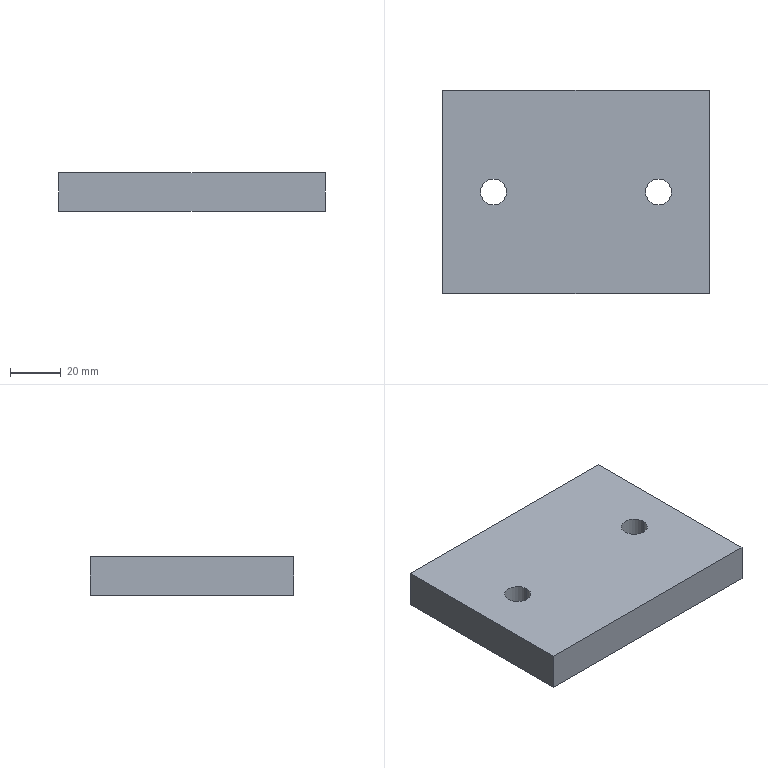Part | SolidWorks | features Extrusion 1, HoleWzd 1 | 1 solid | 10 faces | box 105 x 80 x 15 mm | volume 123549 mm3 | plane 6 | cylinder 4 | commonest cylinder face diameters 10.2 x4
STEP:
#1=CARTESIAN_POINT('',(-27.4,0.,0.));
#2=VERTEX_POINT('',#1);
#3=CARTESIAN_POINT('',(-37.6,0.,0.));
#4=VERTEX_POINT('',#3);
#5=CARTESIAN_POINT('',(-32.5,0.,0.));
#6=DIRECTION('',(0.,0.,-1.));
#7=DIRECTION('',(-1.,0.,0.));
#8=AXIS2_PLACEMENT_3D('',#5,#6,#7);
#9=CIRCLE('',#8,5.1);
#10=EDGE_CURVE('',#2,#4,#9,.T.);
#11=ORIENTED_EDGE('',*,*,#10,.T.);
#12=CARTESIAN_POINT('',(-37.6,0.,15.));
#13=VERTEX_POINT('',#12);
#14=CARTESIAN_POINT('',(-37.6,0.,15.));
#15=DIRECTION('',(0.,0.,1.));
#16=VECTOR('',#15,1000.);
#17=LINE('',#14,#16);
#18=EDGE_CURVE('',#4,#13,#17,.T.);
#19=ORIENTED_EDGE('',*,*,#18,.T.);
#20=CARTESIAN_POINT('',(-27.4,0.,15.));
#21=VERTEX_POINT('',#20);
#22=CARTESIAN_POINT('',(-32.5,0.,15.));
#23=DIRECTION('',(0.,0.,1.));
#24=DIRECTION('',(1.,0.,0.));
#25=AXIS2_PLACEMENT_3D('',#22,#23,#24);
#26=CIRCLE('',#25,5.1);
#27=EDGE_CURVE('',#13,#21,#26,.T.);
#28=ORIENTED_EDGE('',*,*,#27,.T.);
#29=CARTESIAN_POINT('',(-27.4,0.,15.));
#30=DIRECTION('',(0.,0.,1.));
#31=VECTOR('',#30,1000.);
#32=LINE('',#29,#31);
#33=EDGE_CURVE('',#2,#21,#32,.T.);
#34=ORIENTED_EDGE('',*,*,#33,.F.);
#35=EDGE_LOOP('',(#11,#19,#28,#34));
#36=FACE_OUTER_BOUND('',#35,.T.);
#37=CARTESIAN_POINT('',(-32.5,0.,15.));
#38=DIRECTION('',(0.,0.,1.));
#39=DIRECTION('',(1.,0.,0.));
#40=AXIS2_PLACEMENT_3D('',#37,#38,#39);
#41=CYLINDRICAL_SURFACE('',#40,5.1);
#42=ADVANCED_FACE('',(#36),#41,.F.);
#43=CARTESIAN_POINT('',(37.6,0.,0.));
#44=VERTEX_POINT('',#43);
#45=CARTESIAN_POINT('',(27.4,0.,0.));
#46=VERTEX_POINT('',#45);
#47=CARTESIAN_POINT('',(32.5,0.,0.));
#48=DIRECTION('',(0.,0.,-1.));
#49=DIRECTION('',(-1.,0.,0.));
#50=AXIS2_PLACEMENT_3D('',#47,#48,#49);
#51=CIRCLE('',#50,5.1);
#52=EDGE_CURVE('',#44,#46,#51,.T.);
#53=ORIENTED_EDGE('',*,*,#52,.T.);
#54=CARTESIAN_POINT('',(27.4,0.,15.));
#55=VERTEX_POINT('',#54);
#56=CARTESIAN_POINT('',(27.4,0.,15.));
#57=DIRECTION('',(0.,0.,1.));
#58=VECTOR('',#57,1000.);
#59=LINE('',#56,#58);
#60=EDGE_CURVE('',#46,#55,#59,.T.);
#61=ORIENTED_EDGE('',*,*,#60,.T.);
#62=CARTESIAN_POINT('',(37.6,0.,15.));
#63=VERTEX_POINT('',#62);
#64=CARTESIAN_POINT('',(32.5,0.,15.));
#65=DIRECTION('',(0.,0.,1.));
#66=DIRECTION('',(1.,0.,0.));
#67=AXIS2_PLACEMENT_3D('',#64,#65,#66);
#68=CIRCLE('',#67,5.1);
#69=EDGE_CURVE('',#55,#63,#68,.T.);
#70=ORIENTED_EDGE('',*,*,#69,.T.);
#71=CARTESIAN_POINT('',(37.6,0.,15.));
#72=DIRECTION('',(0.,0.,1.));
#73=VECTOR('',#72,1000.);
#74=LINE('',#71,#73);
#75=EDGE_CURVE('',#44,#63,#74,.T.);
#76=ORIENTED_EDGE('',*,*,#75,.F.);
#77=EDGE_LOOP('',(#53,#61,#70,#76));
#78=FACE_OUTER_BOUND('',#77,.T.);
#79=CARTESIAN_POINT('',(32.5,0.,15.));
#80=DIRECTION('',(0.,0.,1.));
#81=DIRECTION('',(1.,0.,0.));
#82=AXIS2_PLACEMENT_3D('',#79,#80,#81);
#83=CYLINDRICAL_SURFACE('',#82,5.1);
#84=ADVANCED_FACE('',(#78),#83,.F.);
#85=CARTESIAN_POINT('',(-52.5,40.,0.));
#86=VERTEX_POINT('',#85);
#87=CARTESIAN_POINT('',(-52.5,-40.,0.));
#88=VERTEX_POINT('',#87);
#89=CARTESIAN_POINT('',(-52.5,40.,0.));
#90=DIRECTION('',(0.,-1.,0.));
#91=VECTOR('',#90,1000.);
#92=LINE('',#89,#91);
#93=EDGE_CURVE('',#86,#88,#92,.T.);
#94=ORIENTED_EDGE('',*,*,#93,.T.);
#95=CARTESIAN_POINT('',(-52.5,-40.,15.));
#96=VERTEX_POINT('',#95);
#97=CARTESIAN_POINT('',(-52.5,-40.,15.));
#98=DIRECTION('',(0.,0.,-1.));
#99=VECTOR('',#98,1000.);
#100=LINE('',#97,#99);
#101=EDGE_CURVE('',#96,#88,#100,.T.);
#102=ORIENTED_EDGE('',*,*,#101,.F.);
#103=CARTESIAN_POINT('',(-52.5,40.,15.));
#104=VERTEX_POINT('',#103);
#105=CARTESIAN_POINT('',(-52.5,40.,15.));
#106=DIRECTION('',(0.,-1.,0.));
#107=VECTOR('',#106,1000.);
#108=LINE('',#105,#107);
#109=EDGE_CURVE('',#104,#96,#108,.T.);
#110=ORIENTED_EDGE('',*,*,#109,.F.);
#111=CARTESIAN_POINT('',(-52.5,40.,15.));
#112=DIRECTION('',(0.,0.,-1.));
#113=VECTOR('',#112,1000.);
#114=LINE('',#111,#113);
#115=EDGE_CURVE('',#104,#86,#114,.T.);
#116=ORIENTED_EDGE('',*,*,#115,.T.);
#117=EDGE_LOOP('',(#94,#102,#110,#116));
#118=FACE_OUTER_BOUND('',#117,.T.);
#119=CARTESIAN_POINT('',(-52.5,40.,15.));
#120=DIRECTION('',(1.,0.,0.));
#121=DIRECTION('',(0.,0.,-1.));
#122=AXIS2_PLACEMENT_3D('',#119,#120,#121);
#123=PLANE('',#122);
#124=ADVANCED_FACE('',(#118),#123,.F.);
#125=CARTESIAN_POINT('',(52.5,-40.,0.));
#126=VERTEX_POINT('',#125);
#127=CARTESIAN_POINT('',(52.5,-40.,0.));
#128=DIRECTION('',(1.,0.,0.));
#129=VECTOR('',#128,1000.);
#130=LINE('',#127,#129);
#131=EDGE_CURVE('',#88,#126,#130,.T.);
#132=ORIENTED_EDGE('',*,*,#131,.T.);
#133=CARTESIAN_POINT('',(52.5,-40.,15.));
#134=VERTEX_POINT('',#133);
#135=CARTESIAN_POINT('',(52.5,-40.,15.));
#136=DIRECTION('',(0.,0.,-1.));
#137=VECTOR('',#136,1000.);
#138=LINE('',#135,#137);
#139=EDGE_CURVE('',#134,#126,#138,.T.);
#140=ORIENTED_EDGE('',*,*,#139,.F.);
#141=CARTESIAN_POINT('',(52.5,-40.,15.));
#142=DIRECTION('',(1.,0.,0.));
#143=VECTOR('',#142,1000.);
#144=LINE('',#141,#143);
#145=EDGE_CURVE('',#96,#134,#144,.T.);
#146=ORIENTED_EDGE('',*,*,#145,.F.);
#147=ORIENTED_EDGE('',*,*,#101,.T.);
#148=EDGE_LOOP('',(#132,#140,#146,#147));
#149=FACE_OUTER_BOUND('',#148,.T.);
#150=CARTESIAN_POINT('',(52.5,-40.,15.));
#151=DIRECTION('',(0.,1.,0.));
#152=DIRECTION('',(-1.,0.,0.));
#153=AXIS2_PLACEMENT_3D('',#150,#151,#152);
#154=PLANE('',#153);
#155=ADVANCED_FACE('',(#149),#154,.F.);
#156=CARTESIAN_POINT('',(52.5,40.,0.));
#157=VERTEX_POINT('',#156);
#158=CARTESIAN_POINT('',(52.5,40.,0.));
#159=DIRECTION('',(0.,1.,0.));
#160=VECTOR('',#159,1000.);
#161=LINE('',#158,#160);
#162=EDGE_CURVE('',#126,#157,#161,.T.);
#163=ORIENTED_EDGE('',*,*,#162,.T.);
#164=CARTESIAN_POINT('',(52.5,40.,15.));
#165=VERTEX_POINT('',#164);
#166=CARTESIAN_POINT('',(52.5,40.,15.));
#167=DIRECTION('',(0.,0.,-1.));
#168=VECTOR('',#167,1000.);
#169=LINE('',#166,#168);
#170=EDGE_CURVE('',#165,#157,#169,.T.);
#171=ORIENTED_EDGE('',*,*,#170,.F.);
#172=CARTESIAN_POINT('',(52.5,40.,15.));
#173=DIRECTION('',(0.,1.,0.));
#174=VECTOR('',#173,1000.);
#175=LINE('',#172,#174);
#176=EDGE_CURVE('',#134,#165,#175,.T.);
#177=ORIENTED_EDGE('',*,*,#176,.F.);
#178=ORIENTED_EDGE('',*,*,#139,.T.);
#179=EDGE_LOOP('',(#163,#171,#177,#178));
#180=FACE_OUTER_BOUND('',#179,.T.);
#181=CARTESIAN_POINT('',(52.5,40.,15.));
#182=DIRECTION('',(-1.,0.,0.));
#183=DIRECTION('',(0.,-1.,0.));
#184=AXIS2_PLACEMENT_3D('',#181,#182,#183);
#185=PLANE('',#184);
#186=ADVANCED_FACE('',(#180),#185,.F.);
#187=CARTESIAN_POINT('',(52.5,40.,0.));
#188=DIRECTION('',(-1.,0.,0.));
#189=VECTOR('',#188,1000.);
#190=LINE('',#187,#189);
#191=EDGE_CURVE('',#157,#86,#190,.T.);
#192=ORIENTED_EDGE('',*,*,#191,.T.);
#193=ORIENTED_EDGE('',*,*,#115,.F.);
#194=CARTESIAN_POINT('',(52.5,40.,15.));
#195=DIRECTION('',(-1.,0.,0.));
#196=VECTOR('',#195,1000.);
#197=LINE('',#194,#196);
#198=EDGE_CURVE('',#165,#104,#197,.T.);
#199=ORIENTED_EDGE('',*,*,#198,.F.);
#200=ORIENTED_EDGE('',*,*,#170,.T.);
#201=EDGE_LOOP('',(#192,#193,#199,#200));
#202=FACE_OUTER_BOUND('',#201,.T.);
#203=CARTESIAN_POINT('',(52.5,40.,15.));
#204=DIRECTION('',(0.,-1.,0.));
#205=DIRECTION('',(1.,0.,0.));
#206=AXIS2_PLACEMENT_3D('',#203,#204,#205);
#207=PLANE('',#206);
#208=ADVANCED_FACE('',(#202),#207,.F.);
#209=CARTESIAN_POINT('',(-32.5,0.,15.));
#210=DIRECTION('',(0.,0.,1.));
#211=DIRECTION('',(1.,0.,0.));
#212=AXIS2_PLACEMENT_3D('',#209,#210,#211);
#213=CIRCLE('',#212,5.1);
#214=EDGE_CURVE('',#21,#13,#213,.T.);
#215=ORIENTED_EDGE('',*,*,#214,.F.);
#216=ORIENTED_EDGE('',*,*,#27,.F.);
#217=EDGE_LOOP('',(#215,#216));
#218=FACE_BOUND('',#217,.T.);
#219=CARTESIAN_POINT('',(32.5,0.,15.));
#220=DIRECTION('',(0.,0.,1.));
#221=DIRECTION('',(1.,0.,0.));
#222=AXIS2_PLACEMENT_3D('',#219,#220,#221);
#223=CIRCLE('',#222,5.1);
#224=EDGE_CURVE('',#63,#55,#223,.T.);
#225=ORIENTED_EDGE('',*,*,#224,.F.);
#226=ORIENTED_EDGE('',*,*,#69,.F.);
#227=EDGE_LOOP('',(#225,#226));
#228=FACE_BOUND('',#227,.T.);
#229=ORIENTED_EDGE('',*,*,#109,.T.);
#230=ORIENTED_EDGE('',*,*,#145,.T.);
#231=ORIENTED_EDGE('',*,*,#176,.T.);
#232=ORIENTED_EDGE('',*,*,#198,.T.);
#233=EDGE_LOOP('',(#229,#230,#231,#232));
#234=FACE_OUTER_BOUND('',#233,.T.);
#235=CARTESIAN_POINT('',(0.,0.,15.));
#236=DIRECTION('',(0.,0.,-1.));
#237=DIRECTION('',(-1.,0.,0.));
#238=AXIS2_PLACEMENT_3D('',#235,#236,#237);
#239=PLANE('',#238);
#240=ADVANCED_FACE('',(#218,#228,#234),#239,.F.);
#241=ORIENTED_EDGE('',*,*,#10,.F.);
#242=CARTESIAN_POINT('',(-32.5,0.,0.));
#243=DIRECTION('',(0.,0.,-1.));
#244=DIRECTION('',(-1.,0.,0.));
#245=AXIS2_PLACEMENT_3D('',#242,#243,#244);
#246=CIRCLE('',#245,5.1);
#247=EDGE_CURVE('',#4,#2,#246,.T.);
#248=ORIENTED_EDGE('',*,*,#247,.F.);
#249=EDGE_LOOP('',(#241,#248));
#250=FACE_BOUND('',#249,.T.);
#251=ORIENTED_EDGE('',*,*,#52,.F.);
#252=CARTESIAN_POINT('',(32.5,0.,0.));
#253=DIRECTION('',(0.,0.,-1.));
#254=DIRECTION('',(-1.,0.,0.));
#255=AXIS2_PLACEMENT_3D('',#252,#253,#254);
#256=CIRCLE('',#255,5.1);
#257=EDGE_CURVE('',#46,#44,#256,.T.);
#258=ORIENTED_EDGE('',*,*,#257,.F.);
#259=EDGE_LOOP('',(#251,#258));
#260=FACE_BOUND('',#259,.T.);
#261=ORIENTED_EDGE('',*,*,#93,.F.);
#262=ORIENTED_EDGE('',*,*,#191,.F.);
#263=ORIENTED_EDGE('',*,*,#162,.F.);
#264=ORIENTED_EDGE('',*,*,#131,.F.);
#265=EDGE_LOOP('',(#261,#262,#263,#264));
#266=FACE_OUTER_BOUND('',#265,.T.);
#267=CARTESIAN_POINT('',(0.,0.,0.));
#268=DIRECTION('',(0.,0.,-1.));
#269=DIRECTION('',(-1.,0.,0.));
#270=AXIS2_PLACEMENT_3D('',#267,#268,#269);
#271=PLANE('',#270);
#272=ADVANCED_FACE('',(#250,#260,#266),#271,.T.);
#273=ORIENTED_EDGE('',*,*,#60,.F.);
#274=ORIENTED_EDGE('',*,*,#257,.T.);
#275=ORIENTED_EDGE('',*,*,#75,.T.);
#276=ORIENTED_EDGE('',*,*,#224,.T.);
#277=EDGE_LOOP('',(#273,#274,#275,#276));
#278=FACE_OUTER_BOUND('',#277,.T.);
#279=CARTESIAN_POINT('',(32.5,0.,15.));
#280=DIRECTION('',(0.,0.,1.));
#281=DIRECTION('',(1.,0.,0.));
#282=AXIS2_PLACEMENT_3D('',#279,#280,#281);
#283=CYLINDRICAL_SURFACE('',#282,5.1);
#284=ADVANCED_FACE('',(#278),#283,.F.);
#285=ORIENTED_EDGE('',*,*,#18,.F.);
#286=ORIENTED_EDGE('',*,*,#247,.T.);
#287=ORIENTED_EDGE('',*,*,#33,.T.);
#288=ORIENTED_EDGE('',*,*,#214,.T.);
#289=EDGE_LOOP('',(#285,#286,#287,#288));
#290=FACE_OUTER_BOUND('',#289,.T.);
#291=CARTESIAN_POINT('',(-32.5,0.,15.));
#292=DIRECTION('',(0.,0.,1.));
#293=DIRECTION('',(1.,0.,0.));
#294=AXIS2_PLACEMENT_3D('',#291,#292,#293);
#295=CYLINDRICAL_SURFACE('',#294,5.1);
#296=ADVANCED_FACE('',(#290),#295,.F.);
#297=CLOSED_SHELL('',(#42,#84,#124,#155,#186,#208,#240,#272,#284,#296));
#298=MANIFOLD_SOLID_BREP('',#297);
#299=CARTESIAN_POINT('',(0.,0.,0.));
#300=DIRECTION('',(0.,0.,1.));
#301=DIRECTION('',(1.,0.,0.));
#302=AXIS2_PLACEMENT_3D('',#299,#300,#301);
#303=(LENGTH_UNIT()NAMED_UNIT(*)SI_UNIT(.MILLI.,.METRE.));
#304=UNCERTAINTY_MEASURE_WITH_UNIT(LENGTH_MEASURE(0.00001),#303,'','');
#305=(NAMED_UNIT(*)PLANE_ANGLE_UNIT()SI_UNIT($,.RADIAN.));
#306=(NAMED_UNIT(*)SI_UNIT($,.STERADIAN.)SOLID_ANGLE_UNIT());
#307=(GEOMETRIC_REPRESENTATION_CONTEXT(3)GLOBAL_UNCERTAINTY_ASSIGNED_CONTEXT((#304))GLOBAL_UNIT_ASSIGNED_CONTEXT((#303,#305,#306))REPRESENTATION_CONTEXT('',''));
#308=ADVANCED_BREP_SHAPE_REPRESENTATION('',(#298,#302),#307);